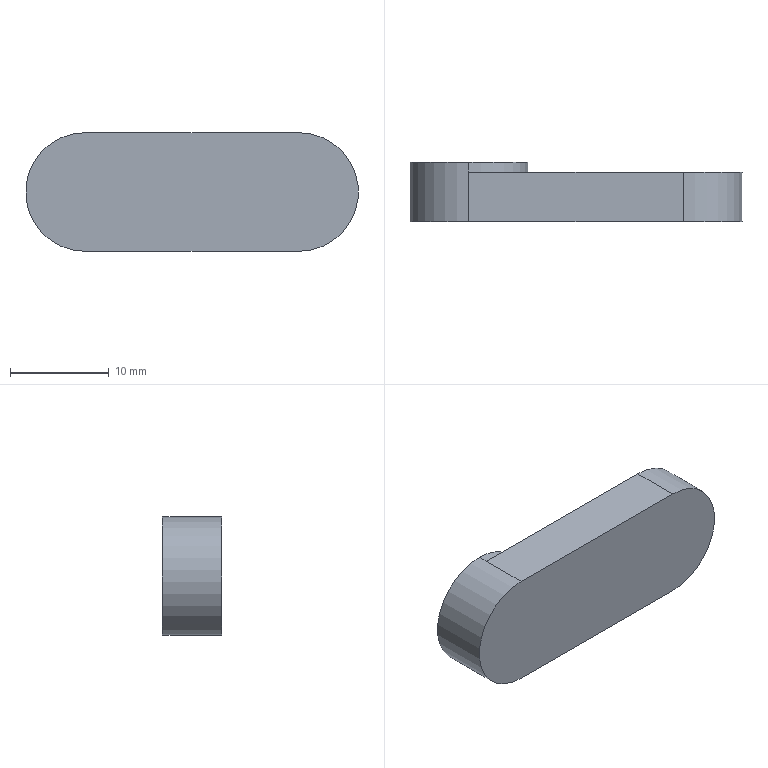Part | STEP file | TYYUTI_Default | 1 solid | 8 faces | box 33.7 x 6 x 12 mm | volume 1981 mm3 | plane 5 | cylinder 3 | commonest cylinder face diameters 12 x3
STEP:
#1=CARTESIAN_POINT('',(0.,0.,0.));
#2=DIRECTION('',(0.,0.,1.));
#3=DIRECTION('',(1.,0.,0.));
#4=AXIS2_PLACEMENT_3D('',#1,#2,#3);
#5=CARTESIAN_POINT('',(-10.85,6.,6.));
#6=VERTEX_POINT('',#5);
#7=CARTESIAN_POINT('',(-10.85,6.,-6.));
#8=VERTEX_POINT('',#7);
#9=CARTESIAN_POINT('',(-10.85,6.,0.));
#10=DIRECTION('',(0.,1.,0.));
#11=DIRECTION('',(0.,0.,1.));
#12=AXIS2_PLACEMENT_3D('',#9,#10,#11);
#13=CIRCLE('',#12,6.);
#14=CARTESIAN_POINT('',(-10.85,5.,0.));
#15=DIRECTION('',(0.,-1.,0.));
#16=DIRECTION('',(0.,0.,-1.));
#17=AXIS2_PLACEMENT_3D('',#14,#15,#16);
#18=CYLINDRICAL_SURFACE('',#17,6.);
#19=CARTESIAN_POINT('',(3.142,-1.));
#20=DIRECTION('',(-1.,0.));
#21=VECTOR('',#20,1.);
#22=LINE('',#19,#21);
#23=(GEOMETRIC_REPRESENTATION_CONTEXT(2)PARAMETRIC_REPRESENTATION_CONTEXT()REPRESENTATION_CONTEXT('',''));
#24=DEFINITIONAL_REPRESENTATION('',(#22),#23);
#25=PCURVE('',#18,#24);
#26=CARTESIAN_POINT('',(-10.85,6.,0.));
#27=DIRECTION('',(0.,1.,0.));
#28=DIRECTION('',(0.,0.,1.));
#29=AXIS2_PLACEMENT_3D('',#26,#27,#28);
#30=PLANE('',#29);
#31=CARTESIAN_POINT('',(0.,0.));
#32=DIRECTION('',(1.,0.));
#33=AXIS2_PLACEMENT_2D('',#31,#32);
#34=CIRCLE('',#33,6.);
#35=(GEOMETRIC_REPRESENTATION_CONTEXT(2)PARAMETRIC_REPRESENTATION_CONTEXT()REPRESENTATION_CONTEXT('',''));
#36=DEFINITIONAL_REPRESENTATION('',(#34),#35);
#37=PCURVE('',#30,#36);
#38=SURFACE_CURVE('',#13,(#25,#37),.PCURVE_S1.);
#39=EDGE_CURVE('',#6,#8,#38,.T.);
#40=ORIENTED_EDGE('',*,*,#39,.F.);
#41=CARTESIAN_POINT('',(-10.85,5.,6.));
#42=VERTEX_POINT('',#41);
#43=CARTESIAN_POINT('',(-10.85,5.,6.));
#44=DIRECTION('',(0.,-1.,0.));
#45=VECTOR('',#44,1.);
#46=LINE('',#43,#45);
#47=CARTESIAN_POINT('',(3.142,0.));
#48=DIRECTION('',(0.,1.));
#49=VECTOR('',#48,1.);
#50=LINE('',#47,#49);
#51=(GEOMETRIC_REPRESENTATION_CONTEXT(2)PARAMETRIC_REPRESENTATION_CONTEXT()REPRESENTATION_CONTEXT('',''));
#52=DEFINITIONAL_REPRESENTATION('',(#50),#51);
#53=PCURVE('',#18,#52);
#54=CARTESIAN_POINT('',(-10.85,5.,0.));
#55=DIRECTION('',(0.,-1.,0.));
#56=DIRECTION('',(0.,0.,-1.));
#57=AXIS2_PLACEMENT_3D('',#54,#55,#56);
#58=CYLINDRICAL_SURFACE('',#57,6.);
#59=CARTESIAN_POINT('',(3.142,0.));
#60=DIRECTION('',(0.,1.));
#61=VECTOR('',#60,1.);
#62=LINE('',#59,#61);
#63=(GEOMETRIC_REPRESENTATION_CONTEXT(2)PARAMETRIC_REPRESENTATION_CONTEXT()REPRESENTATION_CONTEXT('',''));
#64=DEFINITIONAL_REPRESENTATION('',(#62),#63);
#65=PCURVE('',#58,#64);
#66=SURFACE_CURVE('',#46,(#53,#65),.PCURVE_S1.);
#67=EDGE_CURVE('',#6,#42,#66,.T.);
#68=ORIENTED_EDGE('',*,*,#67,.T.);
#69=CARTESIAN_POINT('',(-10.85,5.,-6.));
#70=VERTEX_POINT('',#69);
#71=CARTESIAN_POINT('',(-10.85,5.,0.));
#72=DIRECTION('',(0.,1.,0.));
#73=DIRECTION('',(0.,0.,1.));
#74=AXIS2_PLACEMENT_3D('',#71,#72,#73);
#75=CIRCLE('',#74,6.);
#76=CARTESIAN_POINT('',(3.142,0.));
#77=DIRECTION('',(-1.,0.));
#78=VECTOR('',#77,1.);
#79=LINE('',#76,#78);
#80=(GEOMETRIC_REPRESENTATION_CONTEXT(2)PARAMETRIC_REPRESENTATION_CONTEXT()REPRESENTATION_CONTEXT('',''));
#81=DEFINITIONAL_REPRESENTATION('',(#79),#80);
#82=PCURVE('',#18,#81);
#83=CARTESIAN_POINT('',(10.85,5.,0.));
#84=DIRECTION('',(0.,1.,0.));
#85=DIRECTION('',(0.,0.,1.));
#86=AXIS2_PLACEMENT_3D('',#83,#84,#85);
#87=PLANE('',#86);
#88=CARTESIAN_POINT('',(0.,-21.7));
#89=DIRECTION('',(1.,0.));
#90=AXIS2_PLACEMENT_2D('',#88,#89);
#91=CIRCLE('',#90,6.);
#92=(GEOMETRIC_REPRESENTATION_CONTEXT(2)PARAMETRIC_REPRESENTATION_CONTEXT()REPRESENTATION_CONTEXT('',''));
#93=DEFINITIONAL_REPRESENTATION('',(#91),#92);
#94=PCURVE('',#87,#93);
#95=SURFACE_CURVE('',#75,(#82,#94),.PCURVE_S1.);
#96=EDGE_CURVE('',#42,#70,#95,.T.);
#97=ORIENTED_EDGE('',*,*,#96,.T.);
#98=CARTESIAN_POINT('',(-10.85,5.,-6.));
#99=DIRECTION('',(0.,-1.,0.));
#100=VECTOR('',#99,1.);
#101=LINE('',#98,#100);
#102=CARTESIAN_POINT('',(0.,0.));
#103=DIRECTION('',(0.,1.));
#104=VECTOR('',#103,1.);
#105=LINE('',#102,#104);
#106=(GEOMETRIC_REPRESENTATION_CONTEXT(2)PARAMETRIC_REPRESENTATION_CONTEXT()REPRESENTATION_CONTEXT('',''));
#107=DEFINITIONAL_REPRESENTATION('',(#105),#106);
#108=PCURVE('',#18,#107);
#109=CARTESIAN_POINT('',(6.283,0.));
#110=DIRECTION('',(0.,1.));
#111=VECTOR('',#110,1.);
#112=LINE('',#109,#111);
#113=(GEOMETRIC_REPRESENTATION_CONTEXT(2)PARAMETRIC_REPRESENTATION_CONTEXT()REPRESENTATION_CONTEXT('',''));
#114=DEFINITIONAL_REPRESENTATION('',(#112),#113);
#115=PCURVE('',#58,#114);
#116=SURFACE_CURVE('',#101,(#108,#115),.PCURVE_S1.);
#117=EDGE_CURVE('',#8,#70,#116,.T.);
#118=ORIENTED_EDGE('',*,*,#117,.F.);
#119=EDGE_LOOP('',(#40,#68,#97,#118));
#120=FACE_BOUND('',#119,.T.);
#121=ADVANCED_FACE('',(#120),#18,.T.);
#122=CARTESIAN_POINT('',(10.85,0.,6.));
#123=VERTEX_POINT('',#122);
#124=CARTESIAN_POINT('',(10.85,0.,-6.));
#125=VERTEX_POINT('',#124);
#126=CARTESIAN_POINT('',(10.85,0.,0.));
#127=DIRECTION('',(0.,1.,0.));
#128=DIRECTION('',(0.,0.,1.));
#129=AXIS2_PLACEMENT_3D('',#126,#127,#128);
#130=CIRCLE('',#129,6.);
#131=CARTESIAN_POINT('',(10.85,5.,0.));
#132=DIRECTION('',(0.,-1.,0.));
#133=DIRECTION('',(0.,0.,-1.));
#134=AXIS2_PLACEMENT_3D('',#131,#132,#133);
#135=CYLINDRICAL_SURFACE('',#134,6.);
#136=CARTESIAN_POINT('',(3.142,5.));
#137=DIRECTION('',(-1.,0.));
#138=VECTOR('',#137,1.);
#139=LINE('',#136,#138);
#140=(GEOMETRIC_REPRESENTATION_CONTEXT(2)PARAMETRIC_REPRESENTATION_CONTEXT()REPRESENTATION_CONTEXT('',''));
#141=DEFINITIONAL_REPRESENTATION('',(#139),#140);
#142=PCURVE('',#135,#141);
#143=CARTESIAN_POINT('',(10.85,0.,0.));
#144=DIRECTION('',(0.,1.,0.));
#145=DIRECTION('',(0.,0.,1.));
#146=AXIS2_PLACEMENT_3D('',#143,#144,#145);
#147=PLANE('',#146);
#148=CARTESIAN_POINT('',(0.,0.));
#149=DIRECTION('',(1.,0.));
#150=AXIS2_PLACEMENT_2D('',#148,#149);
#151=CIRCLE('',#150,6.);
#152=(GEOMETRIC_REPRESENTATION_CONTEXT(2)PARAMETRIC_REPRESENTATION_CONTEXT()REPRESENTATION_CONTEXT('',''));
#153=DEFINITIONAL_REPRESENTATION('',(#151),#152);
#154=PCURVE('',#147,#153);
#155=SURFACE_CURVE('',#130,(#142,#154),.PCURVE_S1.);
#156=EDGE_CURVE('',#123,#125,#155,.T.);
#157=ORIENTED_EDGE('',*,*,#156,.T.);
#158=CARTESIAN_POINT('',(10.85,5.,-6.));
#159=VERTEX_POINT('',#158);
#160=CARTESIAN_POINT('',(10.85,5.,-6.));
#161=DIRECTION('',(0.,-1.,0.));
#162=VECTOR('',#161,1.);
#163=LINE('',#160,#162);
#164=CARTESIAN_POINT('',(0.,0.));
#165=DIRECTION('',(0.,1.));
#166=VECTOR('',#165,1.);
#167=LINE('',#164,#166);
#168=(GEOMETRIC_REPRESENTATION_CONTEXT(2)PARAMETRIC_REPRESENTATION_CONTEXT()REPRESENTATION_CONTEXT('',''));
#169=DEFINITIONAL_REPRESENTATION('',(#167),#168);
#170=PCURVE('',#135,#169);
#171=CARTESIAN_POINT('',(10.85,5.,-6.));
#172=DIRECTION('',(0.,0.,1.));
#173=DIRECTION('',(1.,0.,0.));
#174=AXIS2_PLACEMENT_3D('',#171,#172,#173);
#175=PLANE('',#174);
#176=CARTESIAN_POINT('',(0.,0.));
#177=DIRECTION('',(0.,-1.));
#178=VECTOR('',#177,1.);
#179=LINE('',#176,#178);
#180=(GEOMETRIC_REPRESENTATION_CONTEXT(2)PARAMETRIC_REPRESENTATION_CONTEXT()REPRESENTATION_CONTEXT('',''));
#181=DEFINITIONAL_REPRESENTATION('',(#179),#180);
#182=PCURVE('',#175,#181);
#183=SURFACE_CURVE('',#163,(#170,#182),.PCURVE_S1.);
#184=EDGE_CURVE('',#159,#125,#183,.T.);
#185=ORIENTED_EDGE('',*,*,#184,.F.);
#186=CARTESIAN_POINT('',(10.85,5.,6.));
#187=VERTEX_POINT('',#186);
#188=CARTESIAN_POINT('',(10.85,5.,0.));
#189=DIRECTION('',(0.,1.,0.));
#190=DIRECTION('',(0.,0.,1.));
#191=AXIS2_PLACEMENT_3D('',#188,#189,#190);
#192=CIRCLE('',#191,6.);
#193=CARTESIAN_POINT('',(3.142,0.));
#194=DIRECTION('',(-1.,0.));
#195=VECTOR('',#194,1.);
#196=LINE('',#193,#195);
#197=(GEOMETRIC_REPRESENTATION_CONTEXT(2)PARAMETRIC_REPRESENTATION_CONTEXT()REPRESENTATION_CONTEXT('',''));
#198=DEFINITIONAL_REPRESENTATION('',(#196),#197);
#199=PCURVE('',#135,#198);
#200=CARTESIAN_POINT('',(0.,0.));
#201=DIRECTION('',(1.,0.));
#202=AXIS2_PLACEMENT_2D('',#200,#201);
#203=CIRCLE('',#202,6.);
#204=(GEOMETRIC_REPRESENTATION_CONTEXT(2)PARAMETRIC_REPRESENTATION_CONTEXT()REPRESENTATION_CONTEXT('',''));
#205=DEFINITIONAL_REPRESENTATION('',(#203),#204);
#206=PCURVE('',#87,#205);
#207=SURFACE_CURVE('',#192,(#199,#206),.PCURVE_S1.);
#208=EDGE_CURVE('',#187,#159,#207,.T.);
#209=ORIENTED_EDGE('',*,*,#208,.F.);
#210=CARTESIAN_POINT('',(10.85,5.,6.));
#211=DIRECTION('',(0.,-1.,0.));
#212=VECTOR('',#211,1.);
#213=LINE('',#210,#212);
#214=CARTESIAN_POINT('',(3.142,0.));
#215=DIRECTION('',(0.,1.));
#216=VECTOR('',#215,1.);
#217=LINE('',#214,#216);
#218=(GEOMETRIC_REPRESENTATION_CONTEXT(2)PARAMETRIC_REPRESENTATION_CONTEXT()REPRESENTATION_CONTEXT('',''));
#219=DEFINITIONAL_REPRESENTATION('',(#217),#218);
#220=PCURVE('',#135,#219);
#221=CARTESIAN_POINT('',(10.85,5.,6.));
#222=DIRECTION('',(0.,0.,-1.));
#223=DIRECTION('',(-1.,0.,0.));
#224=AXIS2_PLACEMENT_3D('',#221,#222,#223);
#225=PLANE('',#224);
#226=CARTESIAN_POINT('',(0.,0.));
#227=DIRECTION('',(0.,-1.));
#228=VECTOR('',#227,1.);
#229=LINE('',#226,#228);
#230=(GEOMETRIC_REPRESENTATION_CONTEXT(2)PARAMETRIC_REPRESENTATION_CONTEXT()REPRESENTATION_CONTEXT('',''));
#231=DEFINITIONAL_REPRESENTATION('',(#229),#230);
#232=PCURVE('',#225,#231);
#233=SURFACE_CURVE('',#213,(#220,#232),.PCURVE_S1.);
#234=EDGE_CURVE('',#187,#123,#233,.T.);
#235=ORIENTED_EDGE('',*,*,#234,.T.);
#236=EDGE_LOOP('',(#157,#185,#209,#235));
#237=FACE_BOUND('',#236,.T.);
#238=ADVANCED_FACE('',(#237),#135,.T.);
#239=CARTESIAN_POINT('',(-10.85,0.,-6.));
#240=VERTEX_POINT('',#239);
#241=CARTESIAN_POINT('',(10.85,0.,-6.));
#242=DIRECTION('',(-1.,0.,0.));
#243=VECTOR('',#242,1.);
#244=LINE('',#241,#243);
#245=CARTESIAN_POINT('',(0.,-5.));
#246=DIRECTION('',(-1.,0.));
#247=VECTOR('',#246,1.);
#248=LINE('',#245,#247);
#249=(GEOMETRIC_REPRESENTATION_CONTEXT(2)PARAMETRIC_REPRESENTATION_CONTEXT()REPRESENTATION_CONTEXT('',''));
#250=DEFINITIONAL_REPRESENTATION('',(#248),#249);
#251=PCURVE('',#175,#250);
#252=CARTESIAN_POINT('',(-6.,0.));
#253=DIRECTION('',(0.,-1.));
#254=VECTOR('',#253,1.);
#255=LINE('',#252,#254);
#256=(GEOMETRIC_REPRESENTATION_CONTEXT(2)PARAMETRIC_REPRESENTATION_CONTEXT()REPRESENTATION_CONTEXT('',''));
#257=DEFINITIONAL_REPRESENTATION('',(#255),#256);
#258=PCURVE('',#147,#257);
#259=SURFACE_CURVE('',#244,(#251,#258),.PCURVE_S1.);
#260=EDGE_CURVE('',#125,#240,#259,.T.);
#261=ORIENTED_EDGE('',*,*,#260,.T.);
#262=CARTESIAN_POINT('',(-10.85,5.,-6.));
#263=DIRECTION('',(0.,-1.,0.));
#264=VECTOR('',#263,1.);
#265=LINE('',#262,#264);
#266=CARTESIAN_POINT('',(-21.7,0.));
#267=DIRECTION('',(0.,-1.));
#268=VECTOR('',#267,1.);
#269=LINE('',#266,#268);
#270=(GEOMETRIC_REPRESENTATION_CONTEXT(2)PARAMETRIC_REPRESENTATION_CONTEXT()REPRESENTATION_CONTEXT('',''));
#271=DEFINITIONAL_REPRESENTATION('',(#269),#270);
#272=PCURVE('',#175,#271);
#273=CARTESIAN_POINT('',(6.283,0.));
#274=DIRECTION('',(0.,1.));
#275=VECTOR('',#274,1.);
#276=LINE('',#273,#275);
#277=(GEOMETRIC_REPRESENTATION_CONTEXT(2)PARAMETRIC_REPRESENTATION_CONTEXT()REPRESENTATION_CONTEXT('',''));
#278=DEFINITIONAL_REPRESENTATION('',(#276),#277);
#279=PCURVE('',#58,#278);
#280=SURFACE_CURVE('',#265,(#272,#279),.PCURVE_S1.);
#281=EDGE_CURVE('',#70,#240,#280,.T.);
#282=ORIENTED_EDGE('',*,*,#281,.F.);
#283=CARTESIAN_POINT('',(10.85,5.,-6.));
#284=DIRECTION('',(-1.,0.,0.));
#285=VECTOR('',#284,1.);
#286=LINE('',#283,#285);
#287=CARTESIAN_POINT('',(0.,0.));
#288=DIRECTION('',(-1.,0.));
#289=VECTOR('',#288,1.);
#290=LINE('',#287,#289);
#291=(GEOMETRIC_REPRESENTATION_CONTEXT(2)PARAMETRIC_REPRESENTATION_CONTEXT()REPRESENTATION_CONTEXT('',''));
#292=DEFINITIONAL_REPRESENTATION('',(#290),#291);
#293=PCURVE('',#175,#292);
#294=CARTESIAN_POINT('',(-6.,0.));
#295=DIRECTION('',(0.,-1.));
#296=VECTOR('',#295,1.);
#297=LINE('',#294,#296);
#298=(GEOMETRIC_REPRESENTATION_CONTEXT(2)PARAMETRIC_REPRESENTATION_CONTEXT()REPRESENTATION_CONTEXT('',''));
#299=DEFINITIONAL_REPRESENTATION('',(#297),#298);
#300=PCURVE('',#87,#299);
#301=SURFACE_CURVE('',#286,(#293,#300),.PCURVE_S1.);
#302=EDGE_CURVE('',#159,#70,#301,.T.);
#303=ORIENTED_EDGE('',*,*,#302,.F.);
#304=ORIENTED_EDGE('',*,*,#184,.T.);
#305=EDGE_LOOP('',(#261,#282,#303,#304));
#306=FACE_BOUND('',#305,.T.);
#307=ADVANCED_FACE('',(#306),#175,.F.);
#308=ORIENTED_EDGE('',*,*,#67,.F.);
#309=CARTESIAN_POINT('',(-10.85,6.,0.));
#310=DIRECTION('',(0.,1.,0.));
#311=DIRECTION('',(0.,0.,1.));
#312=AXIS2_PLACEMENT_3D('',#309,#310,#311);
#313=CIRCLE('',#312,6.);
#314=CARTESIAN_POINT('',(9.425,-1.));
#315=DIRECTION('',(-1.,0.));
#316=VECTOR('',#315,1.);
#317=LINE('',#314,#316);
#318=(GEOMETRIC_REPRESENTATION_CONTEXT(2)PARAMETRIC_REPRESENTATION_CONTEXT()REPRESENTATION_CONTEXT('',''));
#319=DEFINITIONAL_REPRESENTATION('',(#317),#318);
#320=PCURVE('',#58,#319);
#321=CARTESIAN_POINT('',(0.,0.));
#322=DIRECTION('',(1.,0.));
#323=AXIS2_PLACEMENT_2D('',#321,#322);
#324=CIRCLE('',#323,6.);
#325=(GEOMETRIC_REPRESENTATION_CONTEXT(2)PARAMETRIC_REPRESENTATION_CONTEXT()REPRESENTATION_CONTEXT('',''));
#326=DEFINITIONAL_REPRESENTATION('',(#324),#325);
#327=PCURVE('',#30,#326);
#328=SURFACE_CURVE('',#313,(#320,#327),.PCURVE_S1.);
#329=EDGE_CURVE('',#8,#6,#328,.T.);
#330=ORIENTED_EDGE('',*,*,#329,.F.);
#331=ORIENTED_EDGE('',*,*,#117,.T.);
#332=ORIENTED_EDGE('',*,*,#281,.T.);
#333=CARTESIAN_POINT('',(-10.85,0.,6.));
#334=VERTEX_POINT('',#333);
#335=CARTESIAN_POINT('',(-10.85,0.,0.));
#336=DIRECTION('',(0.,1.,0.));
#337=DIRECTION('',(0.,0.,1.));
#338=AXIS2_PLACEMENT_3D('',#335,#336,#337);
#339=CIRCLE('',#338,6.);
#340=CARTESIAN_POINT('',(9.425,5.));
#341=DIRECTION('',(-1.,0.));
#342=VECTOR('',#341,1.);
#343=LINE('',#340,#342);
#344=(GEOMETRIC_REPRESENTATION_CONTEXT(2)PARAMETRIC_REPRESENTATION_CONTEXT()REPRESENTATION_CONTEXT('',''));
#345=DEFINITIONAL_REPRESENTATION('',(#343),#344);
#346=PCURVE('',#58,#345);
#347=CARTESIAN_POINT('',(0.,-21.7));
#348=DIRECTION('',(1.,0.));
#349=AXIS2_PLACEMENT_2D('',#347,#348);
#350=CIRCLE('',#349,6.);
#351=(GEOMETRIC_REPRESENTATION_CONTEXT(2)PARAMETRIC_REPRESENTATION_CONTEXT()REPRESENTATION_CONTEXT('',''));
#352=DEFINITIONAL_REPRESENTATION('',(#350),#351);
#353=PCURVE('',#147,#352);
#354=SURFACE_CURVE('',#339,(#346,#353),.PCURVE_S1.);
#355=EDGE_CURVE('',#240,#334,#354,.T.);
#356=ORIENTED_EDGE('',*,*,#355,.T.);
#357=CARTESIAN_POINT('',(-10.85,5.,6.));
#358=DIRECTION('',(0.,-1.,0.));
#359=VECTOR('',#358,1.);
#360=LINE('',#357,#359);
#361=CARTESIAN_POINT('',(3.142,0.));
#362=DIRECTION('',(0.,1.));
#363=VECTOR('',#362,1.);
#364=LINE('',#361,#363);
#365=(GEOMETRIC_REPRESENTATION_CONTEXT(2)PARAMETRIC_REPRESENTATION_CONTEXT()REPRESENTATION_CONTEXT('',''));
#366=DEFINITIONAL_REPRESENTATION('',(#364),#365);
#367=PCURVE('',#58,#366);
#368=CARTESIAN_POINT('',(21.7,0.));
#369=DIRECTION('',(0.,-1.));
#370=VECTOR('',#369,1.);
#371=LINE('',#368,#370);
#372=(GEOMETRIC_REPRESENTATION_CONTEXT(2)PARAMETRIC_REPRESENTATION_CONTEXT()REPRESENTATION_CONTEXT('',''));
#373=DEFINITIONAL_REPRESENTATION('',(#371),#372);
#374=PCURVE('',#225,#373);
#375=SURFACE_CURVE('',#360,(#367,#374),.PCURVE_S1.);
#376=EDGE_CURVE('',#42,#334,#375,.T.);
#377=ORIENTED_EDGE('',*,*,#376,.F.);
#378=EDGE_LOOP('',(#308,#330,#331,#332,#356,#377));
#379=FACE_BOUND('',#378,.T.);
#380=ADVANCED_FACE('',(#379),#58,.T.);
#381=CARTESIAN_POINT('',(10.85,0.,6.));
#382=DIRECTION('',(1.,0.,0.));
#383=VECTOR('',#382,1.);
#384=LINE('',#381,#383);
#385=CARTESIAN_POINT('',(0.,-5.));
#386=DIRECTION('',(-1.,0.));
#387=VECTOR('',#386,1.);
#388=LINE('',#385,#387);
#389=(GEOMETRIC_REPRESENTATION_CONTEXT(2)PARAMETRIC_REPRESENTATION_CONTEXT()REPRESENTATION_CONTEXT('',''));
#390=DEFINITIONAL_REPRESENTATION('',(#388),#389);
#391=PCURVE('',#225,#390);
#392=CARTESIAN_POINT('',(6.,0.));
#393=DIRECTION('',(0.,1.));
#394=VECTOR('',#393,1.);
#395=LINE('',#392,#394);
#396=(GEOMETRIC_REPRESENTATION_CONTEXT(2)PARAMETRIC_REPRESENTATION_CONTEXT()REPRESENTATION_CONTEXT('',''));
#397=DEFINITIONAL_REPRESENTATION('',(#395),#396);
#398=PCURVE('',#147,#397);
#399=SURFACE_CURVE('',#384,(#391,#398),.PCURVE_S1.);
#400=EDGE_CURVE('',#334,#123,#399,.T.);
#401=ORIENTED_EDGE('',*,*,#400,.T.);
#402=ORIENTED_EDGE('',*,*,#234,.F.);
#403=CARTESIAN_POINT('',(10.85,5.,6.));
#404=DIRECTION('',(1.,0.,0.));
#405=VECTOR('',#404,1.);
#406=LINE('',#403,#405);
#407=CARTESIAN_POINT('',(0.,0.));
#408=DIRECTION('',(-1.,0.));
#409=VECTOR('',#408,1.);
#410=LINE('',#407,#409);
#411=(GEOMETRIC_REPRESENTATION_CONTEXT(2)PARAMETRIC_REPRESENTATION_CONTEXT()REPRESENTATION_CONTEXT('',''));
#412=DEFINITIONAL_REPRESENTATION('',(#410),#411);
#413=PCURVE('',#225,#412);
#414=CARTESIAN_POINT('',(6.,0.));
#415=DIRECTION('',(0.,1.));
#416=VECTOR('',#415,1.);
#417=LINE('',#414,#416);
#418=(GEOMETRIC_REPRESENTATION_CONTEXT(2)PARAMETRIC_REPRESENTATION_CONTEXT()REPRESENTATION_CONTEXT('',''));
#419=DEFINITIONAL_REPRESENTATION('',(#417),#418);
#420=PCURVE('',#87,#419);
#421=SURFACE_CURVE('',#406,(#413,#420),.PCURVE_S1.);
#422=EDGE_CURVE('',#42,#187,#421,.T.);
#423=ORIENTED_EDGE('',*,*,#422,.F.);
#424=ORIENTED_EDGE('',*,*,#376,.T.);
#425=EDGE_LOOP('',(#401,#402,#423,#424));
#426=FACE_BOUND('',#425,.T.);
#427=ADVANCED_FACE('',(#426),#225,.F.);
#428=ORIENTED_EDGE('',*,*,#96,.F.);
#429=ORIENTED_EDGE('',*,*,#422,.T.);
#430=ORIENTED_EDGE('',*,*,#208,.T.);
#431=ORIENTED_EDGE('',*,*,#302,.T.);
#432=EDGE_LOOP('',(#428,#429,#430,#431));
#433=FACE_BOUND('',#432,.T.);
#434=ADVANCED_FACE('',(#433),#87,.T.);
#435=ORIENTED_EDGE('',*,*,#156,.F.);
#436=ORIENTED_EDGE('',*,*,#400,.F.);
#437=ORIENTED_EDGE('',*,*,#355,.F.);
#438=ORIENTED_EDGE('',*,*,#260,.F.);
#439=EDGE_LOOP('',(#435,#436,#437,#438));
#440=FACE_BOUND('',#439,.T.);
#441=ADVANCED_FACE('',(#440),#147,.F.);
#442=ORIENTED_EDGE('',*,*,#329,.T.);
#443=ORIENTED_EDGE('',*,*,#39,.T.);
#444=EDGE_LOOP('',(#442,#443));
#445=FACE_BOUND('',#444,.T.);
#446=ADVANCED_FACE('',(#445),#30,.T.);
#447=CLOSED_SHELL('',(#121,#238,#307,#380,#427,#434,#441,#446));
#448=MANIFOLD_SOLID_BREP('',#447);
#449=(LENGTH_UNIT()NAMED_UNIT(*)SI_UNIT(.MILLI.,.METRE.));
#450=UNCERTAINTY_MEASURE_WITH_UNIT(LENGTH_MEASURE(0.0000001),#449,'','');
#451=(NAMED_UNIT(*)PLANE_ANGLE_UNIT()SI_UNIT($,.RADIAN.));
#452=(NAMED_UNIT(*)SI_UNIT($,.STERADIAN.)SOLID_ANGLE_UNIT());
#453=(GEOMETRIC_REPRESENTATION_CONTEXT(3)GLOBAL_UNCERTAINTY_ASSIGNED_CONTEXT((#450))GLOBAL_UNIT_ASSIGNED_CONTEXT((#449,#451,#452))REPRESENTATION_CONTEXT('',''));
#454=ADVANCED_BREP_SHAPE_REPRESENTATION('',(#4,#448),#453);